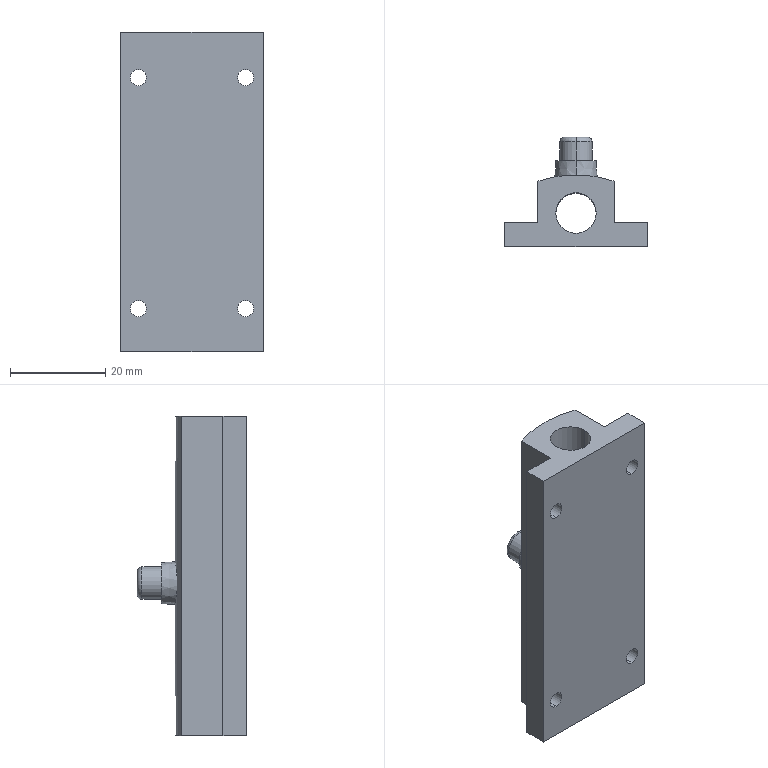Part | SolidWorks | features ICE 4, Extrusion 1, Fillet 1, HoleWzd 1 | 2 solids | 41 faces | box 30 x 23 x 67 mm | volume 16541 mm3 | cylinder 15 | plane 14 | cone 10 | torus 2 | commonest cylinder face diameters 3.4 x8 6.8 x2 7 x2 8.5 x2 50 x1
STEP:
#1=CARTESIAN_POINT('',(-4.25,7.,-33.5));
#2=VERTEX_POINT('',#1);
#3=CARTESIAN_POINT('',(4.25,7.,-33.5));
#4=VERTEX_POINT('',#3);
#5=CARTESIAN_POINT('',(0.,7.,-33.5));
#6=DIRECTION('',(0.,0.,1.));
#7=DIRECTION('',(1.,0.,0.));
#8=AXIS2_PLACEMENT_3D('',#5,#6,#7);
#9=CIRCLE('',#8,4.25);
#10=EDGE_CURVE('',#2,#4,#9,.T.);
#11=ORIENTED_EDGE('',*,*,#10,.F.);
#12=CARTESIAN_POINT('',(-4.25,7.,33.5));
#13=VERTEX_POINT('',#12);
#14=CARTESIAN_POINT('',(-4.25,7.,-33.5));
#15=DIRECTION('',(0.,0.,1.));
#16=VECTOR('',#15,1000.);
#17=LINE('',#14,#16);
#18=EDGE_CURVE('',#2,#13,#17,.T.);
#19=ORIENTED_EDGE('',*,*,#18,.T.);
#20=CARTESIAN_POINT('',(4.25,7.,33.5));
#21=VERTEX_POINT('',#20);
#22=CARTESIAN_POINT('',(0.,7.,33.5));
#23=DIRECTION('',(0.,0.,1.));
#24=DIRECTION('',(1.,0.,0.));
#25=AXIS2_PLACEMENT_3D('',#22,#23,#24);
#26=CIRCLE('',#25,4.25);
#27=EDGE_CURVE('',#13,#21,#26,.T.);
#28=ORIENTED_EDGE('',*,*,#27,.T.);
#29=CARTESIAN_POINT('',(4.25,7.,-33.5));
#30=DIRECTION('',(0.,0.,1.));
#31=VECTOR('',#30,1000.);
#32=LINE('',#29,#31);
#33=EDGE_CURVE('',#4,#21,#32,.T.);
#34=ORIENTED_EDGE('',*,*,#33,.F.);
#35=EDGE_LOOP('',(#11,#19,#28,#34));
#36=FACE_OUTER_BOUND('',#35,.T.);
#37=CARTESIAN_POINT('',(0.,7.,-33.5));
#38=DIRECTION('',(0.,0.,1.));
#39=DIRECTION('',(1.,0.,0.));
#40=AXIS2_PLACEMENT_3D('',#37,#38,#39);
#41=CYLINDRICAL_SURFACE('',#40,4.25);
#42=ADVANCED_FACE('',(#36),#41,.F.);
#43=CARTESIAN_POINT('',(-1.436,11.,-4.692));
#44=VERTEX_POINT('',#43);
#45=CARTESIAN_POINT('',(0.,11.25,-5.));
#46=VERTEX_POINT('',#45);
#47=CARTESIAN_POINT('',(-1.436,11.,-4.692));
#48=CARTESIAN_POINT('',(-1.217,11.079,-4.791));
#49=CARTESIAN_POINT('',(-0.9864,11.141,-4.867));
#50=CARTESIAN_POINT('',(-0.6235,11.206,-4.946));
#51=CARTESIAN_POINT('',(-0.4987,11.222,-4.967));
#52=CARTESIAN_POINT('',(-0.2496,11.245,-4.993));
#53=CARTESIAN_POINT('',(-0.1249,11.25,-5.));
#54=CARTESIAN_POINT('',(0.,11.25,-5.));
#55=B_SPLINE_CURVE_WITH_KNOTS('',3,(#47,#48,#49,#50,#51,#52,#53,#54),.UNSPECIFIED.,.F.,.F.,(4,2,2,4),(0.,0.0007508,0.001126,0.001502),.UNSPECIFIED.);
#56=EDGE_CURVE('',#44,#46,#55,.T.);
#57=ORIENTED_EDGE('',*,*,#56,.T.);
#58=CARTESIAN_POINT('',(0.,18.,-5.));
#59=VERTEX_POINT('',#58);
#60=CARTESIAN_POINT('',(0.,11.,-5.));
#61=DIRECTION('',(0.,1.,0.));
#62=VECTOR('',#61,1000.);
#63=LINE('',#60,#62);
#64=EDGE_CURVE('',#46,#59,#63,.T.);
#65=ORIENTED_EDGE('',*,*,#64,.T.);
#66=CARTESIAN_POINT('',(0.,18.,2.));
#67=VERTEX_POINT('',#66);
#68=CARTESIAN_POINT('',(0.,18.,-1.5));
#69=DIRECTION('',(0.,1.,0.));
#70=DIRECTION('',(0.,0.,1.));
#71=AXIS2_PLACEMENT_3D('',#68,#69,#70);
#72=CIRCLE('',#71,3.5);
#73=EDGE_CURVE('',#59,#67,#72,.T.);
#74=ORIENTED_EDGE('',*,*,#73,.T.);
#75=CARTESIAN_POINT('',(0.,11.25,2.));
#76=VERTEX_POINT('',#75);
#77=CARTESIAN_POINT('',(0.,11.,2.));
#78=DIRECTION('',(0.,1.,0.));
#79=VECTOR('',#78,1000.);
#80=LINE('',#77,#79);
#81=EDGE_CURVE('',#76,#67,#80,.T.);
#82=ORIENTED_EDGE('',*,*,#81,.F.);
#83=CARTESIAN_POINT('',(-1.436,11.,1.692));
#84=VERTEX_POINT('',#83);
#85=CARTESIAN_POINT('',(0.,11.25,2.));
#86=CARTESIAN_POINT('',(-0.2494,11.25,2.));
#87=CARTESIAN_POINT('',(-0.5029,11.227,1.972));
#88=CARTESIAN_POINT('',(-0.9847,11.142,1.868));
#89=CARTESIAN_POINT('',(-1.217,11.079,1.79));
#90=CARTESIAN_POINT('',(-1.436,11.,1.692));
#91=B_SPLINE_CURVE_WITH_KNOTS('',3,(#85,#86,#87,#88,#89,#90),.UNSPECIFIED.,.F.,.F.,(4,2,4),(0.001502,0.002251,0.003),.UNSPECIFIED.);
#92=EDGE_CURVE('',#76,#84,#91,.T.);
#93=ORIENTED_EDGE('',*,*,#92,.T.);
#94=CARTESIAN_POINT('',(0.,11.,-1.5));
#95=DIRECTION('',(0.,1.,0.));
#96=DIRECTION('',(0.,0.,1.));
#97=AXIS2_PLACEMENT_3D('',#94,#95,#96);
#98=CIRCLE('',#97,3.5);
#99=EDGE_CURVE('',#44,#84,#98,.T.);
#100=ORIENTED_EDGE('',*,*,#99,.F.);
#101=EDGE_LOOP('',(#57,#65,#74,#82,#93,#100));
#102=FACE_OUTER_BOUND('',#101,.T.);
#103=CARTESIAN_POINT('',(0.,11.,-1.5));
#104=DIRECTION('',(0.,1.,0.));
#105=DIRECTION('',(0.,0.,1.));
#106=AXIS2_PLACEMENT_3D('',#103,#104,#105);
#107=CYLINDRICAL_SURFACE('',#106,3.5);
#108=ADVANCED_FACE('',(#102),#107,.F.);
#109=CARTESIAN_POINT('',(0.,18.,-5.819));
#110=VERTEX_POINT('',#109);
#111=CARTESIAN_POINT('',(0.,18.,2.819));
#112=VERTEX_POINT('',#111);
#113=CARTESIAN_POINT('',(0.,18.,-1.5));
#114=DIRECTION('',(0.,1.,0.));
#115=DIRECTION('',(0.,0.,1.));
#116=AXIS2_PLACEMENT_3D('',#113,#114,#115);
#117=CIRCLE('',#116,4.319);
#118=EDGE_CURVE('',#110,#112,#117,.T.);
#119=ORIENTED_EDGE('',*,*,#118,.F.);
#120=CARTESIAN_POINT('',(0.,15.,-5.976));
#121=VERTEX_POINT('',#120);
#122=CARTESIAN_POINT('',(0.,5.,-6.5));
#123=DIRECTION('',(0.,-0.9986,-0.05234));
#124=VECTOR('',#123,1000.);
#125=LINE('',#122,#124);
#126=EDGE_CURVE('',#110,#121,#125,.T.);
#127=ORIENTED_EDGE('',*,*,#126,.T.);
#128=CARTESIAN_POINT('',(0.,15.,2.976));
#129=VERTEX_POINT('',#128);
#130=CARTESIAN_POINT('',(0.,15.,-5.976));
#131=CARTESIAN_POINT('',(-0.293,15.,-5.976));
#132=CARTESIAN_POINT('',(-0.5848,14.995,-5.948));
#133=CARTESIAN_POINT('',(-1.166,14.974,-5.833));
#134=CARTESIAN_POINT('',(-1.448,14.96,-5.748));
#135=CARTESIAN_POINT('',(-1.988,14.922,-5.525));
#136=CARTESIAN_POINT('',(-2.25,14.9,-5.386));
#137=CARTESIAN_POINT('',(-2.741,14.85,-5.06));
#138=CARTESIAN_POINT('',(-2.969,14.824,-4.875));
#139=CARTESIAN_POINT('',(-3.388,14.77,-4.459));
#140=CARTESIAN_POINT('',(-3.574,14.744,-4.232));
#141=CARTESIAN_POINT('',(-3.9,14.694,-3.748));
#142=CARTESIAN_POINT('',(-4.041,14.672,-3.487));
#143=CARTESIAN_POINT('',(-4.267,14.633,-2.943));
#144=CARTESIAN_POINT('',(-4.353,14.618,-2.664));
#145=CARTESIAN_POINT('',(-4.468,14.598,-2.088));
#146=CARTESIAN_POINT('',(-4.497,14.592,-1.79));
#147=CARTESIAN_POINT('',(-4.497,14.592,-1.204));
#148=CARTESIAN_POINT('',(-4.468,14.598,-0.9123));
#149=CARTESIAN_POINT('',(-4.352,14.618,-0.3332));
#150=CARTESIAN_POINT('',(-4.265,14.634,-0.04984));
#151=CARTESIAN_POINT('',(-4.039,14.672,0.4895));
#152=CARTESIAN_POINT('',(-3.899,14.695,0.7498));
#153=CARTESIAN_POINT('',(-3.57,14.744,1.238));
#154=CARTESIAN_POINT('',(-3.383,14.771,1.463));
#155=CARTESIAN_POINT('',(-2.969,14.824,1.875));
#156=CARTESIAN_POINT('',(-2.738,14.851,2.063));
#157=CARTESIAN_POINT('',(-2.25,14.9,2.386));
#158=CARTESIAN_POINT('',(-1.992,14.922,2.523));
#159=CARTESIAN_POINT('',(-1.448,14.96,2.748));
#160=CARTESIAN_POINT('',(-1.163,14.975,2.833));
#161=CARTESIAN_POINT('',(-0.589,14.995,2.947));
#162=CARTESIAN_POINT('',(-0.297,15.,2.976));
#163=CARTESIAN_POINT('',(0.,15.,2.976));
#164=B_SPLINE_CURVE_WITH_KNOTS('',3,(#130,#131,#132,#133,#134,#135,#136,#137,#138,#139,#140,#141,#142,#143,#144,#145,#146,#147,#148,#149,#150,#151,#152,#153,#154,#155,#156,#157,#158,#159,#160,#161,#162,#163),.UNSPECIFIED.,.F.,.F.,(4,2,2,2,2,2,2,2,2,2,2,2,2,2,2,2,4),(0.02455,0.02543,0.02631,0.02719,0.02807,0.02894,0.02982,0.0307,0.03158,0.03246,0.03334,0.03421,0.03509,0.03597,0.03685,0.03773,0.03861),.UNSPECIFIED.);
#165=EDGE_CURVE('',#121,#129,#164,.T.);
#166=ORIENTED_EDGE('',*,*,#165,.T.);
#167=CARTESIAN_POINT('',(0.,5.,3.5));
#168=DIRECTION('',(0.,-0.9986,0.05234));
#169=VECTOR('',#168,1000.);
#170=LINE('',#167,#169);
#171=EDGE_CURVE('',#112,#129,#170,.T.);
#172=ORIENTED_EDGE('',*,*,#171,.F.);
#173=EDGE_LOOP('',(#119,#127,#166,#172));
#174=FACE_OUTER_BOUND('',#173,.T.);
#175=CARTESIAN_POINT('',(0.,5.,-1.5));
#176=DIRECTION('',(0.,-1.,0.));
#177=DIRECTION('',(0.,0.,1.));
#178=AXIS2_PLACEMENT_3D('',#175,#176,#177);
#179=CONICAL_SURFACE('',#178,5.,0.05236);
#180=ADVANCED_FACE('',(#174),#179,.T.);
#181=CARTESIAN_POINT('',(-11.25,3.5,-26.2));
#182=VERTEX_POINT('',#181);
#183=CARTESIAN_POINT('',(-11.25,3.5,-22.8));
#184=VERTEX_POINT('',#183);
#185=CARTESIAN_POINT('',(-11.25,3.5,-24.5));
#186=DIRECTION('',(0.,1.,0.));
#187=DIRECTION('',(0.,0.,1.));
#188=AXIS2_PLACEMENT_3D('',#185,#186,#187);
#189=CIRCLE('',#188,1.7);
#190=EDGE_CURVE('',#182,#184,#189,.T.);
#191=ORIENTED_EDGE('',*,*,#190,.F.);
#192=CARTESIAN_POINT('',(-11.25,5.,-27.7));
#193=VERTEX_POINT('',#192);
#194=CARTESIAN_POINT('',(-11.25,5.,-27.7));
#195=DIRECTION('',(0.,0.7071,-0.7071));
#196=VECTOR('',#195,1000.);
#197=LINE('',#194,#196);
#198=EDGE_CURVE('',#182,#193,#197,.T.);
#199=ORIENTED_EDGE('',*,*,#198,.T.);
#200=CARTESIAN_POINT('',(-11.25,5.,-21.3));
#201=VERTEX_POINT('',#200);
#202=CARTESIAN_POINT('',(-11.25,5.,-24.5));
#203=DIRECTION('',(0.,1.,0.));
#204=DIRECTION('',(0.,0.,1.));
#205=AXIS2_PLACEMENT_3D('',#202,#203,#204);
#206=CIRCLE('',#205,3.2);
#207=EDGE_CURVE('',#193,#201,#206,.T.);
#208=ORIENTED_EDGE('',*,*,#207,.T.);
#209=CARTESIAN_POINT('',(-11.25,5.,-21.3));
#210=DIRECTION('',(0.,0.7071,0.7071));
#211=VECTOR('',#210,1000.);
#212=LINE('',#209,#211);
#213=EDGE_CURVE('',#184,#201,#212,.T.);
#214=ORIENTED_EDGE('',*,*,#213,.F.);
#215=EDGE_LOOP('',(#191,#199,#208,#214));
#216=FACE_OUTER_BOUND('',#215,.T.);
#217=CARTESIAN_POINT('',(-11.25,5.,-24.5));
#218=DIRECTION('',(0.,1.,0.));
#219=DIRECTION('',(0.,0.,1.));
#220=AXIS2_PLACEMENT_3D('',#217,#218,#219);
#221=CONICAL_SURFACE('',#220,3.2,0.7854);
#222=ADVANCED_FACE('',(#216),#221,.F.);
#223=CARTESIAN_POINT('',(-11.25,0.,-26.2));
#224=VERTEX_POINT('',#223);
#225=CARTESIAN_POINT('',(-11.25,0.,-22.8));
#226=VERTEX_POINT('',#225);
#227=CARTESIAN_POINT('',(-11.25,0.,-24.5));
#228=DIRECTION('',(0.,1.,0.));
#229=DIRECTION('',(0.,0.,1.));
#230=AXIS2_PLACEMENT_3D('',#227,#228,#229);
#231=CIRCLE('',#230,1.7);
#232=EDGE_CURVE('',#224,#226,#231,.T.);
#233=ORIENTED_EDGE('',*,*,#232,.F.);
#234=CARTESIAN_POINT('',(-11.25,5.,-26.2));
#235=DIRECTION('',(0.,1.,0.));
#236=VECTOR('',#235,1000.);
#237=LINE('',#234,#236);
#238=EDGE_CURVE('',#224,#182,#237,.T.);
#239=ORIENTED_EDGE('',*,*,#238,.T.);
#240=ORIENTED_EDGE('',*,*,#190,.T.);
#241=CARTESIAN_POINT('',(-11.25,5.,-22.8));
#242=DIRECTION('',(0.,1.,0.));
#243=VECTOR('',#242,1000.);
#244=LINE('',#241,#243);
#245=EDGE_CURVE('',#226,#184,#244,.T.);
#246=ORIENTED_EDGE('',*,*,#245,.F.);
#247=EDGE_LOOP('',(#233,#239,#240,#246));
#248=FACE_OUTER_BOUND('',#247,.T.);
#249=CARTESIAN_POINT('',(-11.25,5.,-24.5));
#250=DIRECTION('',(0.,1.,0.));
#251=DIRECTION('',(0.,0.,1.));
#252=AXIS2_PLACEMENT_3D('',#249,#250,#251);
#253=CYLINDRICAL_SURFACE('',#252,1.7);
#254=ADVANCED_FACE('',(#248),#253,.F.);
#255=CARTESIAN_POINT('',(-11.25,3.5,22.3));
#256=VERTEX_POINT('',#255);
#257=CARTESIAN_POINT('',(-11.25,3.5,25.7));
#258=VERTEX_POINT('',#257);
#259=CARTESIAN_POINT('',(-11.25,3.5,24.));
#260=DIRECTION('',(0.,1.,0.));
#261=DIRECTION('',(0.,0.,1.));
#262=AXIS2_PLACEMENT_3D('',#259,#260,#261);
#263=CIRCLE('',#262,1.7);
#264=EDGE_CURVE('',#256,#258,#263,.T.);
#265=ORIENTED_EDGE('',*,*,#264,.F.);
#266=CARTESIAN_POINT('',(-11.25,5.,20.8));
#267=VERTEX_POINT('',#266);
#268=CARTESIAN_POINT('',(-11.25,5.,20.8));
#269=DIRECTION('',(0.,0.7071,-0.7071));
#270=VECTOR('',#269,1000.);
#271=LINE('',#268,#270);
#272=EDGE_CURVE('',#256,#267,#271,.T.);
#273=ORIENTED_EDGE('',*,*,#272,.T.);
#274=CARTESIAN_POINT('',(-11.25,5.,27.2));
#275=VERTEX_POINT('',#274);
#276=CARTESIAN_POINT('',(-11.25,5.,24.));
#277=DIRECTION('',(0.,1.,0.));
#278=DIRECTION('',(0.,0.,1.));
#279=AXIS2_PLACEMENT_3D('',#276,#277,#278);
#280=CIRCLE('',#279,3.2);
#281=EDGE_CURVE('',#267,#275,#280,.T.);
#282=ORIENTED_EDGE('',*,*,#281,.T.);
#283=CARTESIAN_POINT('',(-11.25,5.,27.2));
#284=DIRECTION('',(0.,0.7071,0.7071));
#285=VECTOR('',#284,1000.);
#286=LINE('',#283,#285);
#287=EDGE_CURVE('',#258,#275,#286,.T.);
#288=ORIENTED_EDGE('',*,*,#287,.F.);
#289=EDGE_LOOP('',(#265,#273,#282,#288));
#290=FACE_OUTER_BOUND('',#289,.T.);
#291=CARTESIAN_POINT('',(-11.25,5.,24.));
#292=DIRECTION('',(0.,1.,0.));
#293=DIRECTION('',(0.,0.,1.));
#294=AXIS2_PLACEMENT_3D('',#291,#292,#293);
#295=CONICAL_SURFACE('',#294,3.2,0.7854);
#296=ADVANCED_FACE('',(#290),#295,.F.);
#297=CARTESIAN_POINT('',(-11.25,0.,22.3));
#298=VERTEX_POINT('',#297);
#299=CARTESIAN_POINT('',(-11.25,0.,25.7));
#300=VERTEX_POINT('',#299);
#301=CARTESIAN_POINT('',(-11.25,0.,24.));
#302=DIRECTION('',(0.,1.,0.));
#303=DIRECTION('',(0.,0.,1.));
#304=AXIS2_PLACEMENT_3D('',#301,#302,#303);
#305=CIRCLE('',#304,1.7);
#306=EDGE_CURVE('',#298,#300,#305,.T.);
#307=ORIENTED_EDGE('',*,*,#306,.F.);
#308=CARTESIAN_POINT('',(-11.25,5.,22.3));
#309=DIRECTION('',(0.,1.,0.));
#310=VECTOR('',#309,1000.);
#311=LINE('',#308,#310);
#312=EDGE_CURVE('',#298,#256,#311,.T.);
#313=ORIENTED_EDGE('',*,*,#312,.T.);
#314=ORIENTED_EDGE('',*,*,#264,.T.);
#315=CARTESIAN_POINT('',(-11.25,5.,25.7));
#316=DIRECTION('',(0.,1.,0.));
#317=VECTOR('',#316,1000.);
#318=LINE('',#315,#317);
#319=EDGE_CURVE('',#300,#258,#318,.T.);
#320=ORIENTED_EDGE('',*,*,#319,.F.);
#321=EDGE_LOOP('',(#307,#313,#314,#320));
#322=FACE_OUTER_BOUND('',#321,.T.);
#323=CARTESIAN_POINT('',(-11.25,5.,24.));
#324=DIRECTION('',(0.,1.,0.));
#325=DIRECTION('',(0.,0.,1.));
#326=AXIS2_PLACEMENT_3D('',#323,#324,#325);
#327=CYLINDRICAL_SURFACE('',#326,1.7);
#328=ADVANCED_FACE('',(#322),#327,.F.);
#329=CARTESIAN_POINT('',(11.25,3.5,22.3));
#330=VERTEX_POINT('',#329);
#331=CARTESIAN_POINT('',(11.25,3.5,25.7));
#332=VERTEX_POINT('',#331);
#333=CARTESIAN_POINT('',(11.25,3.5,24.));
#334=DIRECTION('',(0.,1.,0.));
#335=DIRECTION('',(0.,0.,1.));
#336=AXIS2_PLACEMENT_3D('',#333,#334,#335);
#337=CIRCLE('',#336,1.7);
#338=EDGE_CURVE('',#330,#332,#337,.T.);
#339=ORIENTED_EDGE('',*,*,#338,.F.);
#340=CARTESIAN_POINT('',(11.25,5.,20.8));
#341=VERTEX_POINT('',#340);
#342=CARTESIAN_POINT('',(11.25,5.,20.8));
#343=DIRECTION('',(0.,0.7071,-0.7071));
#344=VECTOR('',#343,1000.);
#345=LINE('',#342,#344);
#346=EDGE_CURVE('',#330,#341,#345,.T.);
#347=ORIENTED_EDGE('',*,*,#346,.T.);
#348=CARTESIAN_POINT('',(11.25,5.,27.2));
#349=VERTEX_POINT('',#348);
#350=CARTESIAN_POINT('',(11.25,5.,24.));
#351=DIRECTION('',(0.,1.,0.));
#352=DIRECTION('',(0.,0.,1.));
#353=AXIS2_PLACEMENT_3D('',#350,#351,#352);
#354=CIRCLE('',#353,3.2);
#355=EDGE_CURVE('',#341,#349,#354,.T.);
#356=ORIENTED_EDGE('',*,*,#355,.T.);
#357=CARTESIAN_POINT('',(11.25,5.,27.2));
#358=DIRECTION('',(0.,0.7071,0.7071));
#359=VECTOR('',#358,1000.);
#360=LINE('',#357,#359);
#361=EDGE_CURVE('',#332,#349,#360,.T.);
#362=ORIENTED_EDGE('',*,*,#361,.F.);
#363=EDGE_LOOP('',(#339,#347,#356,#362));
#364=FACE_OUTER_BOUND('',#363,.T.);
#365=CARTESIAN_POINT('',(11.25,5.,24.));
#366=DIRECTION('',(0.,1.,0.));
#367=DIRECTION('',(0.,0.,1.));
#368=AXIS2_PLACEMENT_3D('',#365,#366,#367);
#369=CONICAL_SURFACE('',#368,3.2,0.7854);
#370=ADVANCED_FACE('',(#364),#369,.F.);
#371=CARTESIAN_POINT('',(11.25,0.,22.3));
#372=VERTEX_POINT('',#371);
#373=CARTESIAN_POINT('',(11.25,0.,25.7));
#374=VERTEX_POINT('',#373);
#375=CARTESIAN_POINT('',(11.25,0.,24.));
#376=DIRECTION('',(0.,1.,0.));
#377=DIRECTION('',(0.,0.,1.));
#378=AXIS2_PLACEMENT_3D('',#375,#376,#377);
#379=CIRCLE('',#378,1.7);
#380=EDGE_CURVE('',#372,#374,#379,.T.);
#381=ORIENTED_EDGE('',*,*,#380,.F.);
#382=CARTESIAN_POINT('',(11.25,5.,22.3));
#383=DIRECTION('',(0.,1.,0.));
#384=VECTOR('',#383,1000.);
#385=LINE('',#382,#384);
#386=EDGE_CURVE('',#372,#330,#385,.T.);
#387=ORIENTED_EDGE('',*,*,#386,.T.);
#388=ORIENTED_EDGE('',*,*,#338,.T.);
#389=CARTESIAN_POINT('',(11.25,5.,25.7));
#390=DIRECTION('',(0.,1.,0.));
#391=VECTOR('',#390,1000.);
#392=LINE('',#389,#391);
#393=EDGE_CURVE('',#374,#332,#392,.T.);
#394=ORIENTED_EDGE('',*,*,#393,.F.);
#395=EDGE_LOOP('',(#381,#387,#388,#394));
#396=FACE_OUTER_BOUND('',#395,.T.);
#397=CARTESIAN_POINT('',(11.25,5.,24.));
#398=DIRECTION('',(0.,1.,0.));
#399=DIRECTION('',(0.,0.,1.));
#400=AXIS2_PLACEMENT_3D('',#397,#398,#399);
#401=CYLINDRICAL_SURFACE('',#400,1.7);
#402=ADVANCED_FACE('',(#396),#401,.F.);
#403=CARTESIAN_POINT('',(11.25,3.5,-26.2));
#404=VERTEX_POINT('',#403);
#405=CARTESIAN_POINT('',(11.25,3.5,-22.8));
#406=VERTEX_POINT('',#405);
#407=CARTESIAN_POINT('',(11.25,3.5,-24.5));
#408=DIRECTION('',(0.,1.,0.));
#409=DIRECTION('',(0.,0.,1.));
#410=AXIS2_PLACEMENT_3D('',#407,#408,#409);
#411=CIRCLE('',#410,1.7);
#412=EDGE_CURVE('',#404,#406,#411,.T.);
#413=ORIENTED_EDGE('',*,*,#412,.F.);
#414=CARTESIAN_POINT('',(11.25,5.,-27.7));
#415=VERTEX_POINT('',#414);
#416=CARTESIAN_POINT('',(11.25,5.,-27.7));
#417=DIRECTION('',(0.,0.7071,-0.7071));
#418=VECTOR('',#417,1000.);
#419=LINE('',#416,#418);
#420=EDGE_CURVE('',#404,#415,#419,.T.);
#421=ORIENTED_EDGE('',*,*,#420,.T.);
#422=CARTESIAN_POINT('',(11.25,5.,-21.3));
#423=VERTEX_POINT('',#422);
#424=CARTESIAN_POINT('',(11.25,5.,-24.5));
#425=DIRECTION('',(0.,1.,0.));
#426=DIRECTION('',(0.,0.,1.));
#427=AXIS2_PLACEMENT_3D('',#424,#425,#426);
#428=CIRCLE('',#427,3.2);
#429=EDGE_CURVE('',#415,#423,#428,.T.);
#430=ORIENTED_EDGE('',*,*,#429,.T.);
#431=CARTESIAN_POINT('',(11.25,5.,-21.3));
#432=DIRECTION('',(0.,0.7071,0.7071));
#433=VECTOR('',#432,1000.);
#434=LINE('',#431,#433);
#435=EDGE_CURVE('',#406,#423,#434,.T.);
#436=ORIENTED_EDGE('',*,*,#435,.F.);
#437=EDGE_LOOP('',(#413,#421,#430,#436));
#438=FACE_OUTER_BOUND('',#437,.T.);
#439=CARTESIAN_POINT('',(11.25,5.,-24.5));
#440=DIRECTION('',(0.,1.,0.));
#441=DIRECTION('',(0.,0.,1.));
#442=AXIS2_PLACEMENT_3D('',#439,#440,#441);
#443=CONICAL_SURFACE('',#442,3.2,0.7854);
#444=ADVANCED_FACE('',(#438),#443,.F.);
#445=CARTESIAN_POINT('',(11.25,0.,-26.2));
#446=VERTEX_POINT('',#445);
#447=CARTESIAN_POINT('',(11.25,0.,-22.8));
#448=VERTEX_POINT('',#447);
#449=CARTESIAN_POINT('',(11.25,0.,-24.5));
#450=DIRECTION('',(0.,1.,0.));
#451=DIRECTION('',(0.,0.,1.));
#452=AXIS2_PLACEMENT_3D('',#449,#450,#451);
#453=CIRCLE('',#452,1.7);
#454=EDGE_CURVE('',#446,#448,#453,.T.);
#455=ORIENTED_EDGE('',*,*,#454,.F.);
#456=CARTESIAN_POINT('',(11.25,5.,-26.2));
#457=DIRECTION('',(0.,1.,0.));
#458=VECTOR('',#457,1000.);
#459=LINE('',#456,#458);
#460=EDGE_CURVE('',#446,#404,#459,.T.);
#461=ORIENTED_EDGE('',*,*,#460,.T.);
#462=ORIENTED_EDGE('',*,*,#412,.T.);
#463=CARTESIAN_POINT('',(11.25,5.,-22.8));
#464=DIRECTION('',(0.,1.,0.));
#465=VECTOR('',#464,1000.);
#466=LINE('',#463,#465);
#467=EDGE_CURVE('',#448,#406,#466,.T.);
#468=ORIENTED_EDGE('',*,*,#467,.F.);
#469=EDGE_LOOP('',(#455,#461,#462,#468));
#470=FACE_OUTER_BOUND('',#469,.T.);
#471=CARTESIAN_POINT('',(11.25,5.,-24.5));
#472=DIRECTION('',(0.,1.,0.));
#473=DIRECTION('',(0.,0.,1.));
#474=AXIS2_PLACEMENT_3D('',#471,#472,#473);
#475=CYLINDRICAL_SURFACE('',#474,1.7);
#476=ADVANCED_FACE('',(#470),#475,.F.);
#477=CARTESIAN_POINT('',(-1.436,11.,-33.5));
#478=DIRECTION('',(0.,0.,1.));
#479=VECTOR('',#478,1000.);
#480=LINE('',#477,#479);
#481=EDGE_CURVE('',#44,#84,#480,.T.);
#482=ORIENTED_EDGE('',*,*,#481,.F.);
#483=ORIENTED_EDGE('',*,*,#99,.T.);
#484=EDGE_LOOP('',(#482,#483));
#485=FACE_OUTER_BOUND('',#484,.T.);
#486=CARTESIAN_POINT('',(0.,11.,-1.5));
#487=DIRECTION('',(0.,1.,0.));
#488=DIRECTION('',(0.,0.,1.));
#489=AXIS2_PLACEMENT_3D('',#486,#487,#488);
#490=PLANE('',#489);
#491=ADVANCED_FACE('',(#485),#490,.T.);
#492=CARTESIAN_POINT('',(8.,13.685,-33.5));
#493=VERTEX_POINT('',#492);
#494=CARTESIAN_POINT('',(-8.,13.685,-33.5));
#495=VERTEX_POINT('',#494);
#496=CARTESIAN_POINT('',(0.,-10.,-33.5));
#497=DIRECTION('',(0.,0.,1.));
#498=DIRECTION('',(-1.,0.,0.));
#499=AXIS2_PLACEMENT_3D('',#496,#497,#498);
#500=CIRCLE('',#499,25.);
#501=EDGE_CURVE('',#493,#495,#500,.T.);
#502=ORIENTED_EDGE('',*,*,#501,.T.);
#503=CARTESIAN_POINT('',(-8.,13.685,33.5));
#504=VERTEX_POINT('',#503);
#505=CARTESIAN_POINT('',(-8.,13.685,33.5));
#506=DIRECTION('',(0.,0.,-1.));
#507=VECTOR('',#506,1000.);
#508=LINE('',#505,#507);
#509=EDGE_CURVE('',#504,#495,#508,.T.);
#510=ORIENTED_EDGE('',*,*,#509,.F.);
#511=CARTESIAN_POINT('',(8.,13.685,33.5));
#512=VERTEX_POINT('',#511);
#513=CARTESIAN_POINT('',(0.,-10.,33.5));
#514=DIRECTION('',(0.,0.,1.));
#515=DIRECTION('',(-1.,0.,0.));
#516=AXIS2_PLACEMENT_3D('',#513,#514,#515);
#517=CIRCLE('',#516,25.);
#518=EDGE_CURVE('',#512,#504,#517,.T.);
#519=ORIENTED_EDGE('',*,*,#518,.F.);
#520=CARTESIAN_POINT('',(8.,13.685,33.5));
#521=DIRECTION('',(0.,0.,-1.));
#522=VECTOR('',#521,1000.);
#523=LINE('',#520,#522);
#524=EDGE_CURVE('',#512,#493,#523,.T.);
#525=ORIENTED_EDGE('',*,*,#524,.T.);
#526=EDGE_LOOP('',(#502,#510,#519,#525));
#527=FACE_OUTER_BOUND('',#526,.T.);
#528=CARTESIAN_POINT('',(0.,15.,2.976));
#529=CARTESIAN_POINT('',(0.297,15.,2.976));
#530=CARTESIAN_POINT('',(0.589,14.995,2.947));
#531=CARTESIAN_POINT('',(1.164,14.975,2.833));
#532=CARTESIAN_POINT('',(1.449,14.959,2.747));
#533=CARTESIAN_POINT('',(1.993,14.922,2.523));
#534=CARTESIAN_POINT('',(2.251,14.9,2.386));
#535=CARTESIAN_POINT('',(2.739,14.851,2.062));
#536=CARTESIAN_POINT('',(2.97,14.824,1.874));
#537=CARTESIAN_POINT('',(3.384,14.771,1.462));
#538=CARTESIAN_POINT('',(3.57,14.744,1.237));
#539=CARTESIAN_POINT('',(3.9,14.695,0.7484));
#540=CARTESIAN_POINT('',(4.04,14.672,0.4884));
#541=CARTESIAN_POINT('',(4.265,14.634,-0.05062));
#542=CARTESIAN_POINT('',(4.352,14.618,-0.3337));
#543=CARTESIAN_POINT('',(4.468,14.598,-0.9132));
#544=CARTESIAN_POINT('',(4.497,14.592,-1.205));
#545=CARTESIAN_POINT('',(4.497,14.592,-1.791));
#546=CARTESIAN_POINT('',(4.468,14.598,-2.089));
#547=CARTESIAN_POINT('',(4.352,14.618,-2.665));
#548=CARTESIAN_POINT('',(4.267,14.633,-2.945));
#549=CARTESIAN_POINT('',(4.04,14.672,-3.488));
#550=CARTESIAN_POINT('',(3.899,14.695,-3.75));
#551=CARTESIAN_POINT('',(3.573,14.744,-4.234));
#552=CARTESIAN_POINT('',(3.385,14.771,-4.461));
#553=CARTESIAN_POINT('',(2.967,14.824,-4.877));
#554=CARTESIAN_POINT('',(2.74,14.851,-5.061));
#555=CARTESIAN_POINT('',(2.254,14.899,-5.384));
#556=CARTESIAN_POINT('',(1.99,14.922,-5.524));
#557=CARTESIAN_POINT('',(1.447,14.96,-5.748));
#558=CARTESIAN_POINT('',(1.167,14.974,-5.832));
#559=CARTESIAN_POINT('',(0.5907,14.995,-5.947));
#560=CARTESIAN_POINT('',(0.2931,15.,-5.976));
#561=CARTESIAN_POINT('',(0.,15.,-5.976));
#562=B_SPLINE_CURVE_WITH_KNOTS('',3,(#528,#529,#530,#531,#532,#533,#534,#535,#536,#537,#538,#539,#540,#541,#542,#543,#544,#545,#546,#547,#548,#549,#550,#551,#552,#553,#554,#555,#556,#557,#558,#559,#560,#561),.UNSPECIFIED.,.F.,.F.,(4,2,2,2,2,2,2,2,2,2,2,2,2,2,2,2,4),(0.01049,0.01137,0.01225,0.01313,0.01401,0.01489,0.01577,0.01664,0.01752,0.0184,0.01928,0.02016,0.02104,0.02192,0.02279,0.02367,0.02455),.UNSPECIFIED.);
#563=EDGE_CURVE('',#129,#121,#562,.T.);
#564=ORIENTED_EDGE('',*,*,#563,.F.);
#565=ORIENTED_EDGE('',*,*,#165,.F.);
#566=EDGE_LOOP('',(#564,#565));
#567=FACE_BOUND('',#566,.T.);
#568=CARTESIAN_POINT('',(0.,-10.,33.5));
#569=DIRECTION('',(0.,0.,-1.));
#570=DIRECTION('',(-1.,0.,0.));
#571=AXIS2_PLACEMENT_3D('',#568,#569,#570);
#572=CYLINDRICAL_SURFACE('',#571,25.);
#573=ADVANCED_FACE('',(#527,#567),#572,.T.);
#574=CARTESIAN_POINT('',(15.,0.,-33.5));
#575=VERTEX_POINT('',#574);
#576=CARTESIAN_POINT('',(15.,5.,-33.5));
#577=VERTEX_POINT('',#576);
#578=CARTESIAN_POINT('',(15.,5.,-33.5));
#579=DIRECTION('',(0.,1.,0.));
#580=VECTOR('',#579,1000.);
#581=LINE('',#578,#580);
#582=EDGE_CURVE('',#575,#577,#581,.T.);
#583=ORIENTED_EDGE('',*,*,#582,.T.);
#584=CARTESIAN_POINT('',(15.,5.,33.5));
#585=VERTEX_POINT('',#584);
#586=CARTESIAN_POINT('',(15.,5.,33.5));
#587=DIRECTION('',(0.,0.,-1.));
#588=VECTOR('',#587,1000.);
#589=LINE('',#586,#588);
#590=EDGE_CURVE('',#585,#577,#589,.T.);
#591=ORIENTED_EDGE('',*,*,#590,.F.);
#592=CARTESIAN_POINT('',(15.,0.,33.5));
#593=VERTEX_POINT('',#592);
#594=CARTESIAN_POINT('',(15.,5.,33.5));
#595=DIRECTION('',(0.,1.,0.));
#596=VECTOR('',#595,1000.);
#597=LINE('',#594,#596);
#598=EDGE_CURVE('',#593,#585,#597,.T.);
#599=ORIENTED_EDGE('',*,*,#598,.F.);
#600=CARTESIAN_POINT('',(15.,0.,33.5));
#601=DIRECTION('',(0.,0.,-1.));
#602=VECTOR('',#601,1000.);
#603=LINE('',#600,#602);
#604=EDGE_CURVE('',#593,#575,#603,.T.);
#605=ORIENTED_EDGE('',*,*,#604,.T.);
#606=EDGE_LOOP('',(#583,#591,#599,#605));
#607=FACE_OUTER_BOUND('',#606,.T.);
#608=CARTESIAN_POINT('',(15.,5.,33.5));
#609=DIRECTION('',(-1.,0.,0.));
#610=DIRECTION('',(0.,-1.,0.));
#611=AXIS2_PLACEMENT_3D('',#608,#609,#610);
#612=PLANE('',#611);
#613=ADVANCED_FACE('',(#607),#612,.F.);
#614=CARTESIAN_POINT('',(11.25,5.,24.));
#615=DIRECTION('',(0.,1.,0.));
#616=DIRECTION('',(0.,0.,1.));
#617=AXIS2_PLACEMENT_3D('',#614,#615,#616);
#618=CIRCLE('',#617,3.2);
#619=EDGE_CURVE('',#349,#341,#618,.T.);
#620=ORIENTED_EDGE('',*,*,#619,.F.);
#621=ORIENTED_EDGE('',*,*,#355,.F.);
#622=EDGE_LOOP('',(#620,#621));
#623=FACE_BOUND('',#622,.T.);
#624=CARTESIAN_POINT('',(11.25,5.,-24.5));
#625=DIRECTION('',(0.,1.,0.));
#626=DIRECTION('',(0.,0.,1.));
#627=AXIS2_PLACEMENT_3D('',#624,#625,#626);
#628=CIRCLE('',#627,3.2);
#629=EDGE_CURVE('',#423,#415,#628,.T.);
#630=ORIENTED_EDGE('',*,*,#629,.F.);
#631=ORIENTED_EDGE('',*,*,#429,.F.);
#632=EDGE_LOOP('',(#630,#631));
#633=FACE_BOUND('',#632,.T.);
#634=CARTESIAN_POINT('',(8.,5.,-33.5));
#635=VERTEX_POINT('',#634);
#636=CARTESIAN_POINT('',(15.,5.,-33.5));
#637=DIRECTION('',(-1.,0.,0.));
#638=VECTOR('',#637,1000.);
#639=LINE('',#636,#638);
#640=EDGE_CURVE('',#577,#635,#639,.T.);
#641=ORIENTED_EDGE('',*,*,#640,.T.);
#642=CARTESIAN_POINT('',(8.,5.,33.5));
#643=VERTEX_POINT('',#642);
#644=CARTESIAN_POINT('',(8.,5.,33.5));
#645=DIRECTION('',(0.,0.,-1.));
#646=VECTOR('',#645,1000.);
#647=LINE('',#644,#646);
#648=EDGE_CURVE('',#643,#635,#647,.T.);
#649=ORIENTED_EDGE('',*,*,#648,.F.);
#650=CARTESIAN_POINT('',(15.,5.,33.5));
#651=DIRECTION('',(-1.,0.,0.));
#652=VECTOR('',#651,1000.);
#653=LINE('',#650,#652);
#654=EDGE_CURVE('',#585,#643,#653,.T.);
#655=ORIENTED_EDGE('',*,*,#654,.F.);
#656=ORIENTED_EDGE('',*,*,#590,.T.);
#657=EDGE_LOOP('',(#641,#649,#655,#656));
#658=FACE_OUTER_BOUND('',#657,.T.);
#659=CARTESIAN_POINT('',(15.,5.,33.5));
#660=DIRECTION('',(0.,-1.,0.));
#661=DIRECTION('',(1.,0.,0.));
#662=AXIS2_PLACEMENT_3D('',#659,#660,#661);
#663=PLANE('',#662);
#664=ADVANCED_FACE('',(#623,#633,#658),#663,.F.);
#665=CARTESIAN_POINT('',(8.,5.,-33.5));
#666=DIRECTION('',(0.,1.,0.));
#667=VECTOR('',#666,1000.);
#668=LINE('',#665,#667);
#669=EDGE_CURVE('',#635,#493,#668,.T.);
#670=ORIENTED_EDGE('',*,*,#669,.T.);
#671=ORIENTED_EDGE('',*,*,#524,.F.);
#672=CARTESIAN_POINT('',(8.,5.,33.5));
#673=DIRECTION('',(0.,1.,0.));
#674=VECTOR('',#673,1000.);
#675=LINE('',#672,#674);
#676=EDGE_CURVE('',#643,#512,#675,.T.);
#677=ORIENTED_EDGE('',*,*,#676,.F.);
#678=ORIENTED_EDGE('',*,*,#648,.T.);
#679=EDGE_LOOP('',(#670,#671,#677,#678));
#680=FACE_OUTER_BOUND('',#679,.T.);
#681=CARTESIAN_POINT('',(8.,5.,33.5));
#682=DIRECTION('',(-1.,0.,0.));
#683=DIRECTION('',(0.,0.,1.));
#684=AXIS2_PLACEMENT_3D('',#681,#682,#683);
#685=PLANE('',#684);
#686=ADVANCED_FACE('',(#680),#685,.F.);
#687=CARTESIAN_POINT('',(-8.,5.,-33.5));
#688=VERTEX_POINT('',#687);
#689=CARTESIAN_POINT('',(-8.,5.,-33.5));
#690=DIRECTION('',(0.,-1.,0.));
#691=VECTOR('',#690,1000.);
#692=LINE('',#689,#691);
#693=EDGE_CURVE('',#495,#688,#692,.T.);
#694=ORIENTED_EDGE('',*,*,#693,.T.);
#695=CARTESIAN_POINT('',(-8.,5.,33.5));
#696=VERTEX_POINT('',#695);
#697=CARTESIAN_POINT('',(-8.,5.,33.5));
#698=DIRECTION('',(0.,0.,-1.));
#699=VECTOR('',#698,1000.);
#700=LINE('',#697,#699);
#701=EDGE_CURVE('',#696,#688,#700,.T.);
#702=ORIENTED_EDGE('',*,*,#701,.F.);
#703=CARTESIAN_POINT('',(-8.,5.,33.5));
#704=DIRECTION('',(0.,-1.,0.));
#705=VECTOR('',#704,1000.);
#706=LINE('',#703,#705);
#707=EDGE_CURVE('',#504,#696,#706,.T.);
#708=ORIENTED_EDGE('',*,*,#707,.F.);
#709=ORIENTED_EDGE('',*,*,#509,.T.);
#710=EDGE_LOOP('',(#694,#702,#708,#709));
#711=FACE_OUTER_BOUND('',#710,.T.);
#712=CARTESIAN_POINT('',(-8.,5.,33.5));
#713=DIRECTION('',(1.,0.,0.));
#714=DIRECTION('',(0.,0.,-1.));
#715=AXIS2_PLACEMENT_3D('',#712,#713,#714);
#716=PLANE('',#715);
#717=ADVANCED_FACE('',(#711),#716,.F.);
#718=CARTESIAN_POINT('',(-11.25,5.,-24.5));
#719=DIRECTION('',(0.,1.,0.));
#720=DIRECTION('',(0.,0.,1.));
#721=AXIS2_PLACEMENT_3D('',#718,#719,#720);
#722=CIRCLE('',#721,3.2);
#723=EDGE_CURVE('',#201,#193,#722,.T.);
#724=ORIENTED_EDGE('',*,*,#723,.F.);
#725=ORIENTED_EDGE('',*,*,#207,.F.);
#726=EDGE_LOOP('',(#724,#725));
#727=FACE_BOUND('',#726,.T.);
#728=CARTESIAN_POINT('',(-11.25,5.,24.));
#729=DIRECTION('',(0.,1.,0.));
#730=DIRECTION('',(0.,0.,1.));
#731=AXIS2_PLACEMENT_3D('',#728,#729,#730);
#732=CIRCLE('',#731,3.2);
#733=EDGE_CURVE('',#275,#267,#732,.T.);
#734=ORIENTED_EDGE('',*,*,#733,.F.);
#735=ORIENTED_EDGE('',*,*,#281,.F.);
#736=EDGE_LOOP('',(#734,#735));
#737=FACE_BOUND('',#736,.T.);
#738=CARTESIAN_POINT('',(-15.,5.,-33.5));
#739=VERTEX_POINT('',#738);
#740=CARTESIAN_POINT('',(-15.,5.,-33.5));
#741=DIRECTION('',(-1.,0.,0.));
#742=VECTOR('',#741,1000.);
#743=LINE('',#740,#742);
#744=EDGE_CURVE('',#688,#739,#743,.T.);
#745=ORIENTED_EDGE('',*,*,#744,.T.);
#746=CARTESIAN_POINT('',(-15.,5.,33.5));
#747=VERTEX_POINT('',#746);
#748=CARTESIAN_POINT('',(-15.,5.,33.5));
#749=DIRECTION('',(0.,0.,-1.));
#750=VECTOR('',#749,1000.);
#751=LINE('',#748,#750);
#752=EDGE_CURVE('',#747,#739,#751,.T.);
#753=ORIENTED_EDGE('',*,*,#752,.F.);
#754=CARTESIAN_POINT('',(-15.,5.,33.5));
#755=DIRECTION('',(-1.,0.,0.));
#756=VECTOR('',#755,1000.);
#757=LINE('',#754,#756);
#758=EDGE_CURVE('',#696,#747,#757,.T.);
#759=ORIENTED_EDGE('',*,*,#758,.F.);
#760=ORIENTED_EDGE('',*,*,#701,.T.);
#761=EDGE_LOOP('',(#745,#753,#759,#760));
#762=FACE_OUTER_BOUND('',#761,.T.);
#763=CARTESIAN_POINT('',(-15.,5.,33.5));
#764=DIRECTION('',(0.,-1.,0.));
#765=DIRECTION('',(0.,0.,-1.));
#766=AXIS2_PLACEMENT_3D('',#763,#764,#765);
#767=PLANE('',#766);
#768=ADVANCED_FACE('',(#727,#737,#762),#767,.F.);
#769=CARTESIAN_POINT('',(-15.,0.,-33.5));
#770=VERTEX_POINT('',#769);
#771=CARTESIAN_POINT('',(-15.,5.,-33.5));
#772=DIRECTION('',(0.,-1.,0.));
#773=VECTOR('',#772,1000.);
#774=LINE('',#771,#773);
#775=EDGE_CURVE('',#739,#770,#774,.T.);
#776=ORIENTED_EDGE('',*,*,#775,.T.);
#777=CARTESIAN_POINT('',(-15.,0.,33.5));
#778=VERTEX_POINT('',#777);
#779=CARTESIAN_POINT('',(-15.,0.,33.5));
#780=DIRECTION('',(0.,0.,-1.));
#781=VECTOR('',#780,1000.);
#782=LINE('',#779,#781);
#783=EDGE_CURVE('',#778,#770,#782,.T.);
#784=ORIENTED_EDGE('',*,*,#783,.F.);
#785=CARTESIAN_POINT('',(-15.,5.,33.5));
#786=DIRECTION('',(0.,-1.,0.));
#787=VECTOR('',#786,1000.);
#788=LINE('',#785,#787);
#789=EDGE_CURVE('',#747,#778,#788,.T.);
#790=ORIENTED_EDGE('',*,*,#789,.F.);
#791=ORIENTED_EDGE('',*,*,#752,.T.);
#792=EDGE_LOOP('',(#776,#784,#790,#791));
#793=FACE_OUTER_BOUND('',#792,.T.);
#794=CARTESIAN_POINT('',(-15.,5.,33.5));
#795=DIRECTION('',(1.,0.,0.));
#796=DIRECTION('',(0.,0.,-1.));
#797=AXIS2_PLACEMENT_3D('',#794,#795,#796);
#798=PLANE('',#797);
#799=ADVANCED_FACE('',(#793),#798,.F.);
#800=CARTESIAN_POINT('',(-11.25,0.,-24.5));
#801=DIRECTION('',(0.,1.,0.));
#802=DIRECTION('',(0.,0.,1.));
#803=AXIS2_PLACEMENT_3D('',#800,#801,#802);
#804=CIRCLE('',#803,1.7);
#805=EDGE_CURVE('',#226,#224,#804,.T.);
#806=ORIENTED_EDGE('',*,*,#805,.T.);
#807=ORIENTED_EDGE('',*,*,#232,.T.);
#808=EDGE_LOOP('',(#806,#807));
#809=FACE_BOUND('',#808,.T.);
#810=CARTESIAN_POINT('',(-11.25,0.,24.));
#811=DIRECTION('',(0.,1.,0.));
#812=DIRECTION('',(0.,0.,1.));
#813=AXIS2_PLACEMENT_3D('',#810,#811,#812);
#814=CIRCLE('',#813,1.7);
#815=EDGE_CURVE('',#300,#298,#814,.T.);
#816=ORIENTED_EDGE('',*,*,#815,.T.);
#817=ORIENTED_EDGE('',*,*,#306,.T.);
#818=EDGE_LOOP('',(#816,#817));
#819=FACE_BOUND('',#818,.T.);
#820=CARTESIAN_POINT('',(11.25,0.,24.));
#821=DIRECTION('',(0.,1.,0.));
#822=DIRECTION('',(0.,0.,1.));
#823=AXIS2_PLACEMENT_3D('',#820,#821,#822);
#824=CIRCLE('',#823,1.7);
#825=EDGE_CURVE('',#374,#372,#824,.T.);
#826=ORIENTED_EDGE('',*,*,#825,.T.);
#827=ORIENTED_EDGE('',*,*,#380,.T.);
#828=EDGE_LOOP('',(#826,#827));
#829=FACE_BOUND('',#828,.T.);
#830=CARTESIAN_POINT('',(11.25,0.,-24.5));
#831=DIRECTION('',(0.,1.,0.));
#832=DIRECTION('',(0.,0.,1.));
#833=AXIS2_PLACEMENT_3D('',#830,#831,#832);
#834=CIRCLE('',#833,1.7);
#835=EDGE_CURVE('',#448,#446,#834,.T.);
#836=ORIENTED_EDGE('',*,*,#835,.T.);
#837=ORIENTED_EDGE('',*,*,#454,.T.);
#838=EDGE_LOOP('',(#836,#837));
#839=FACE_BOUND('',#838,.T.);
#840=CARTESIAN_POINT('',(-15.,0.,-33.5));
#841=DIRECTION('',(1.,0.,0.));
#842=VECTOR('',#841,1000.);
#843=LINE('',#840,#842);
#844=EDGE_CURVE('',#770,#575,#843,.T.);
#845=ORIENTED_EDGE('',*,*,#844,.T.);
#846=ORIENTED_EDGE('',*,*,#604,.F.);
#847=CARTESIAN_POINT('',(-15.,0.,33.5));
#848=DIRECTION('',(1.,0.,0.));
#849=VECTOR('',#848,1000.);
#850=LINE('',#847,#849);
#851=EDGE_CURVE('',#778,#593,#850,.T.);
#852=ORIENTED_EDGE('',*,*,#851,.F.);
#853=ORIENTED_EDGE('',*,*,#783,.T.);
#854=EDGE_LOOP('',(#845,#846,#852,#853));
#855=FACE_OUTER_BOUND('',#854,.T.);
#856=CARTESIAN_POINT('',(-15.,0.,33.5));
#857=DIRECTION('',(0.,1.,0.));
#858=DIRECTION('',(-1.,0.,0.));
#859=AXIS2_PLACEMENT_3D('',#856,#857,#858);
#860=PLANE('',#859);
#861=ADVANCED_FACE('',(#809,#819,#829,#839,#855),#860,.F.);
#862=CARTESIAN_POINT('',(0.,7.,33.5));
#863=DIRECTION('',(0.,0.,1.));
#864=DIRECTION('',(1.,0.,0.));
#865=AXIS2_PLACEMENT_3D('',#862,#863,#864);
#866=CIRCLE('',#865,4.25);
#867=EDGE_CURVE('',#21,#13,#866,.T.);
#868=ORIENTED_EDGE('',*,*,#867,.F.);
#869=ORIENTED_EDGE('',*,*,#27,.F.);
#870=EDGE_LOOP('',(#868,#869));
#871=FACE_BOUND('',#870,.T.);
#872=ORIENTED_EDGE('',*,*,#598,.T.);
#873=ORIENTED_EDGE('',*,*,#654,.T.);
#874=ORIENTED_EDGE('',*,*,#676,.T.);
#875=ORIENTED_EDGE('',*,*,#518,.T.);
#876=ORIENTED_EDGE('',*,*,#707,.T.);
#877=ORIENTED_EDGE('',*,*,#758,.T.);
#878=ORIENTED_EDGE('',*,*,#789,.T.);
#879=ORIENTED_EDGE('',*,*,#851,.T.);
#880=EDGE_LOOP('',(#872,#873,#874,#875,#876,#877,#878,#879));
#881=FACE_OUTER_BOUND('',#880,.T.);
#882=CARTESIAN_POINT('',(0.,-10.,33.5));
#883=DIRECTION('',(0.,0.,-1.));
#884=DIRECTION('',(-1.,0.,0.));
#885=AXIS2_PLACEMENT_3D('',#882,#883,#884);
#886=PLANE('',#885);
#887=ADVANCED_FACE('',(#871,#881),#886,.F.);
#888=CARTESIAN_POINT('',(0.,7.,-33.5));
#889=DIRECTION('',(0.,0.,1.));
#890=DIRECTION('',(1.,0.,0.));
#891=AXIS2_PLACEMENT_3D('',#888,#889,#890);
#892=CIRCLE('',#891,4.25);
#893=EDGE_CURVE('',#4,#2,#892,.T.);
#894=ORIENTED_EDGE('',*,*,#893,.T.);
#895=ORIENTED_EDGE('',*,*,#10,.T.);
#896=EDGE_LOOP('',(#894,#895));
#897=FACE_BOUND('',#896,.T.);
#898=ORIENTED_EDGE('',*,*,#582,.F.);
#899=ORIENTED_EDGE('',*,*,#844,.F.);
#900=ORIENTED_EDGE('',*,*,#775,.F.);
#901=ORIENTED_EDGE('',*,*,#744,.F.);
#902=ORIENTED_EDGE('',*,*,#693,.F.);
#903=ORIENTED_EDGE('',*,*,#501,.F.);
#904=ORIENTED_EDGE('',*,*,#669,.F.);
#905=ORIENTED_EDGE('',*,*,#640,.F.);
#906=EDGE_LOOP('',(#898,#899,#900,#901,#902,#903,#904,#905));
#907=FACE_OUTER_BOUND('',#906,.T.);
#908=CARTESIAN_POINT('',(0.,-10.,-33.5));
#909=DIRECTION('',(0.,0.,-1.));
#910=DIRECTION('',(-1.,0.,0.));
#911=AXIS2_PLACEMENT_3D('',#908,#909,#910);
#912=PLANE('',#911);
#913=ADVANCED_FACE('',(#897,#907),#912,.T.);
#914=ORIENTED_EDGE('',*,*,#460,.F.);
#915=ORIENTED_EDGE('',*,*,#835,.F.);
#916=ORIENTED_EDGE('',*,*,#467,.T.);
#917=CARTESIAN_POINT('',(11.25,3.5,-24.5));
#918=DIRECTION('',(0.,1.,0.));
#919=DIRECTION('',(0.,0.,1.));
#920=AXIS2_PLACEMENT_3D('',#917,#918,#919);
#921=CIRCLE('',#920,1.7);
#922=EDGE_CURVE('',#406,#404,#921,.T.);
#923=ORIENTED_EDGE('',*,*,#922,.T.);
#924=EDGE_LOOP('',(#914,#915,#916,#923));
#925=FACE_OUTER_BOUND('',#924,.T.);
#926=CARTESIAN_POINT('',(11.25,5.,-24.5));
#927=DIRECTION('',(0.,1.,0.));
#928=DIRECTION('',(0.,0.,1.));
#929=AXIS2_PLACEMENT_3D('',#926,#927,#928);
#930=CYLINDRICAL_SURFACE('',#929,1.7);
#931=ADVANCED_FACE('',(#925),#930,.F.);
#932=ORIENTED_EDGE('',*,*,#420,.F.);
#933=ORIENTED_EDGE('',*,*,#922,.F.);
#934=ORIENTED_EDGE('',*,*,#435,.T.);
#935=ORIENTED_EDGE('',*,*,#629,.T.);
#936=EDGE_LOOP('',(#932,#933,#934,#935));
#937=FACE_OUTER_BOUND('',#936,.T.);
#938=CARTESIAN_POINT('',(11.25,5.,-24.5));
#939=DIRECTION('',(0.,1.,0.));
#940=DIRECTION('',(0.,0.,1.));
#941=AXIS2_PLACEMENT_3D('',#938,#939,#940);
#942=CONICAL_SURFACE('',#941,3.2,0.7854);
#943=ADVANCED_FACE('',(#937),#942,.F.);
#944=ORIENTED_EDGE('',*,*,#386,.F.);
#945=ORIENTED_EDGE('',*,*,#825,.F.);
#946=ORIENTED_EDGE('',*,*,#393,.T.);
#947=CARTESIAN_POINT('',(11.25,3.5,24.));
#948=DIRECTION('',(0.,1.,0.));
#949=DIRECTION('',(0.,0.,1.));
#950=AXIS2_PLACEMENT_3D('',#947,#948,#949);
#951=CIRCLE('',#950,1.7);
#952=EDGE_CURVE('',#332,#330,#951,.T.);
#953=ORIENTED_EDGE('',*,*,#952,.T.);
#954=EDGE_LOOP('',(#944,#945,#946,#953));
#955=FACE_OUTER_BOUND('',#954,.T.);
#956=CARTESIAN_POINT('',(11.25,5.,24.));
#957=DIRECTION('',(0.,1.,0.));
#958=DIRECTION('',(0.,0.,1.));
#959=AXIS2_PLACEMENT_3D('',#956,#957,#958);
#960=CYLINDRICAL_SURFACE('',#959,1.7);
#961=ADVANCED_FACE('',(#955),#960,.F.);
#962=ORIENTED_EDGE('',*,*,#346,.F.);
#963=ORIENTED_EDGE('',*,*,#952,.F.);
#964=ORIENTED_EDGE('',*,*,#361,.T.);
#965=ORIENTED_EDGE('',*,*,#619,.T.);
#966=EDGE_LOOP('',(#962,#963,#964,#965));
#967=FACE_OUTER_BOUND('',#966,.T.);
#968=CARTESIAN_POINT('',(11.25,5.,24.));
#969=DIRECTION('',(0.,1.,0.));
#970=DIRECTION('',(0.,0.,1.));
#971=AXIS2_PLACEMENT_3D('',#968,#969,#970);
#972=CONICAL_SURFACE('',#971,3.2,0.7854);
#973=ADVANCED_FACE('',(#967),#972,.F.);
#974=ORIENTED_EDGE('',*,*,#312,.F.);
#975=ORIENTED_EDGE('',*,*,#815,.F.);
#976=ORIENTED_EDGE('',*,*,#319,.T.);
#977=CARTESIAN_POINT('',(-11.25,3.5,24.));
#978=DIRECTION('',(0.,1.,0.));
#979=DIRECTION('',(0.,0.,1.));
#980=AXIS2_PLACEMENT_3D('',#977,#978,#979);
#981=CIRCLE('',#980,1.7);
#982=EDGE_CURVE('',#258,#256,#981,.T.);
#983=ORIENTED_EDGE('',*,*,#982,.T.);
#984=EDGE_LOOP('',(#974,#975,#976,#983));
#985=FACE_OUTER_BOUND('',#984,.T.);
#986=CARTESIAN_POINT('',(-11.25,5.,24.));
#987=DIRECTION('',(0.,1.,0.));
#988=DIRECTION('',(0.,0.,1.));
#989=AXIS2_PLACEMENT_3D('',#986,#987,#988);
#990=CYLINDRICAL_SURFACE('',#989,1.7);
#991=ADVANCED_FACE('',(#985),#990,.F.);
#992=ORIENTED_EDGE('',*,*,#272,.F.);
#993=ORIENTED_EDGE('',*,*,#982,.F.);
#994=ORIENTED_EDGE('',*,*,#287,.T.);
#995=ORIENTED_EDGE('',*,*,#733,.T.);
#996=EDGE_LOOP('',(#992,#993,#994,#995));
#997=FACE_OUTER_BOUND('',#996,.T.);
#998=CARTESIAN_POINT('',(-11.25,5.,24.));
#999=DIRECTION('',(0.,1.,0.));
#1000=DIRECTION('',(0.,0.,1.));
#1001=AXIS2_PLACEMENT_3D('',#998,#999,#1000);
#1002=CONICAL_SURFACE('',#1001,3.2,0.7854);
#1003=ADVANCED_FACE('',(#997),#1002,.F.);
#1004=ORIENTED_EDGE('',*,*,#238,.F.);
#1005=ORIENTED_EDGE('',*,*,#805,.F.);
#1006=ORIENTED_EDGE('',*,*,#245,.T.);
#1007=CARTESIAN_POINT('',(-11.25,3.5,-24.5));
#1008=DIRECTION('',(0.,1.,0.));
#1009=DIRECTION('',(0.,0.,1.));
#1010=AXIS2_PLACEMENT_3D('',#1007,#1008,#1009);
#1011=CIRCLE('',#1010,1.7);
#1012=EDGE_CURVE('',#184,#182,#1011,.T.);
#1013=ORIENTED_EDGE('',*,*,#1012,.T.);
#1014=EDGE_LOOP('',(#1004,#1005,#1006,#1013));
#1015=FACE_OUTER_BOUND('',#1014,.T.);
#1016=CARTESIAN_POINT('',(-11.25,5.,-24.5));
#1017=DIRECTION('',(0.,1.,0.));
#1018=DIRECTION('',(0.,0.,1.));
#1019=AXIS2_PLACEMENT_3D('',#1016,#1017,#1018);
#1020=CYLINDRICAL_SURFACE('',#1019,1.7);
#1021=ADVANCED_FACE('',(#1015),#1020,.F.);
#1022=ORIENTED_EDGE('',*,*,#198,.F.);
#1023=ORIENTED_EDGE('',*,*,#1012,.F.);
#1024=ORIENTED_EDGE('',*,*,#213,.T.);
#1025=ORIENTED_EDGE('',*,*,#723,.T.);
#1026=EDGE_LOOP('',(#1022,#1023,#1024,#1025));
#1027=FACE_OUTER_BOUND('',#1026,.T.);
#1028=CARTESIAN_POINT('',(-11.25,5.,-24.5));
#1029=DIRECTION('',(0.,1.,0.));
#1030=DIRECTION('',(0.,0.,1.));
#1031=AXIS2_PLACEMENT_3D('',#1028,#1029,#1030);
#1032=CONICAL_SURFACE('',#1031,3.2,0.7854);
#1033=ADVANCED_FACE('',(#1027),#1032,.F.);
#1034=ORIENTED_EDGE('',*,*,#126,.F.);
#1035=CARTESIAN_POINT('',(0.,18.,-1.5));
#1036=DIRECTION('',(0.,1.,0.));
#1037=DIRECTION('',(0.,0.,1.));
#1038=AXIS2_PLACEMENT_3D('',#1035,#1036,#1037);
#1039=CIRCLE('',#1038,4.319);
#1040=EDGE_CURVE('',#112,#110,#1039,.T.);
#1041=ORIENTED_EDGE('',*,*,#1040,.F.);
#1042=ORIENTED_EDGE('',*,*,#171,.T.);
#1043=ORIENTED_EDGE('',*,*,#563,.T.);
#1044=EDGE_LOOP('',(#1034,#1041,#1042,#1043));
#1045=FACE_OUTER_BOUND('',#1044,.T.);
#1046=CARTESIAN_POINT('',(0.,5.,-1.5));
#1047=DIRECTION('',(0.,-1.,0.));
#1048=DIRECTION('',(0.,0.,1.));
#1049=AXIS2_PLACEMENT_3D('',#1046,#1047,#1048);
#1050=CONICAL_SURFACE('',#1049,5.,0.05236);
#1051=ADVANCED_FACE('',(#1045),#1050,.T.);
#1052=CARTESIAN_POINT('',(0.,18.,-1.5));
#1053=DIRECTION('',(0.,1.,0.));
#1054=DIRECTION('',(0.,0.,1.));
#1055=AXIS2_PLACEMENT_3D('',#1052,#1053,#1054);
#1056=CIRCLE('',#1055,3.5);
#1057=EDGE_CURVE('',#67,#59,#1056,.T.);
#1058=ORIENTED_EDGE('',*,*,#1057,.F.);
#1059=ORIENTED_EDGE('',*,*,#73,.F.);
#1060=EDGE_LOOP('',(#1058,#1059));
#1061=FACE_BOUND('',#1060,.T.);
#1062=ORIENTED_EDGE('',*,*,#1040,.T.);
#1063=ORIENTED_EDGE('',*,*,#118,.T.);
#1064=EDGE_LOOP('',(#1062,#1063));
#1065=FACE_OUTER_BOUND('',#1064,.T.);
#1066=CARTESIAN_POINT('',(0.,18.,-1.5));
#1067=DIRECTION('',(0.,1.,0.));
#1068=DIRECTION('',(0.,0.,1.));
#1069=AXIS2_PLACEMENT_3D('',#1066,#1067,#1068);
#1070=PLANE('',#1069);
#1071=ADVANCED_FACE('',(#1061,#1065),#1070,.T.);
#1072=ORIENTED_EDGE('',*,*,#64,.F.);
#1073=CARTESIAN_POINT('',(1.436,11.,-4.692));
#1074=VERTEX_POINT('',#1073);
#1075=CARTESIAN_POINT('',(0.,11.25,-5.));
#1076=CARTESIAN_POINT('',(0.2494,11.25,-5.));
#1077=CARTESIAN_POINT('',(0.5029,11.227,-4.972));
#1078=CARTESIAN_POINT('',(0.9847,11.142,-4.868));
#1079=CARTESIAN_POINT('',(1.217,11.079,-4.79));
#1080=CARTESIAN_POINT('',(1.436,11.,-4.692));
#1081=B_SPLINE_CURVE_WITH_KNOTS('',3,(#1075,#1076,#1077,#1078,#1079,#1080),.UNSPECIFIED.,.F.,.F.,(4,2,4),(0.001502,0.002251,0.003),.UNSPECIFIED.);
#1082=EDGE_CURVE('',#46,#1074,#1081,.T.);
#1083=ORIENTED_EDGE('',*,*,#1082,.T.);
#1084=CARTESIAN_POINT('',(1.436,11.,1.692));
#1085=VERTEX_POINT('',#1084);
#1086=CARTESIAN_POINT('',(0.,11.,-1.5));
#1087=DIRECTION('',(0.,1.,0.));
#1088=DIRECTION('',(0.,0.,1.));
#1089=AXIS2_PLACEMENT_3D('',#1086,#1087,#1088);
#1090=CIRCLE('',#1089,3.5);
#1091=EDGE_CURVE('',#1085,#1074,#1090,.T.);
#1092=ORIENTED_EDGE('',*,*,#1091,.F.);
#1093=CARTESIAN_POINT('',(1.436,11.,1.692));
#1094=CARTESIAN_POINT('',(1.217,11.079,1.791));
#1095=CARTESIAN_POINT('',(0.9864,11.141,1.867));
#1096=CARTESIAN_POINT('',(0.6235,11.206,1.946));
#1097=CARTESIAN_POINT('',(0.4987,11.222,1.967));
#1098=CARTESIAN_POINT('',(0.2496,11.245,1.993));
#1099=CARTESIAN_POINT('',(0.1249,11.25,2.));
#1100=CARTESIAN_POINT('',(0.,11.25,2.));
#1101=B_SPLINE_CURVE_WITH_KNOTS('',3,(#1093,#1094,#1095,#1096,#1097,#1098,#1099,#1100),.UNSPECIFIED.,.F.,.F.,(4,2,2,4),(0.,0.0007508,0.001126,0.001502),.UNSPECIFIED.);
#1102=EDGE_CURVE('',#1085,#76,#1101,.T.);
#1103=ORIENTED_EDGE('',*,*,#1102,.T.);
#1104=ORIENTED_EDGE('',*,*,#81,.T.);
#1105=ORIENTED_EDGE('',*,*,#1057,.T.);
#1106=EDGE_LOOP('',(#1072,#1083,#1092,#1103,#1104,#1105));
#1107=FACE_OUTER_BOUND('',#1106,.T.);
#1108=CARTESIAN_POINT('',(0.,11.,-1.5));
#1109=DIRECTION('',(0.,1.,0.));
#1110=DIRECTION('',(0.,0.,1.));
#1111=AXIS2_PLACEMENT_3D('',#1108,#1109,#1110);
#1112=CYLINDRICAL_SURFACE('',#1111,3.5);
#1113=ADVANCED_FACE('',(#1107),#1112,.F.);
#1114=CARTESIAN_POINT('',(1.436,11.,-33.5));
#1115=DIRECTION('',(0.,0.,-1.));
#1116=VECTOR('',#1115,1000.);
#1117=LINE('',#1114,#1116);
#1118=EDGE_CURVE('',#1085,#1074,#1117,.T.);
#1119=ORIENTED_EDGE('',*,*,#1118,.F.);
#1120=ORIENTED_EDGE('',*,*,#1091,.T.);
#1121=EDGE_LOOP('',(#1119,#1120));
#1122=FACE_OUTER_BOUND('',#1121,.T.);
#1123=CARTESIAN_POINT('',(0.,11.,-1.5));
#1124=DIRECTION('',(0.,1.,0.));
#1125=DIRECTION('',(0.,0.,1.));
#1126=AXIS2_PLACEMENT_3D('',#1123,#1124,#1125);
#1127=PLANE('',#1126);
#1128=ADVANCED_FACE('',(#1122),#1127,.T.);
#1129=ORIENTED_EDGE('',*,*,#18,.F.);
#1130=ORIENTED_EDGE('',*,*,#893,.F.);
#1131=ORIENTED_EDGE('',*,*,#33,.T.);
#1132=ORIENTED_EDGE('',*,*,#867,.T.);
#1133=EDGE_LOOP('',(#1129,#1130,#1131,#1132));
#1134=FACE_OUTER_BOUND('',#1133,.T.);
#1135=ORIENTED_EDGE('',*,*,#481,.T.);
#1136=ORIENTED_EDGE('',*,*,#92,.F.);
#1137=ORIENTED_EDGE('',*,*,#1102,.F.);
#1138=ORIENTED_EDGE('',*,*,#1118,.T.);
#1139=ORIENTED_EDGE('',*,*,#1082,.F.);
#1140=ORIENTED_EDGE('',*,*,#56,.F.);
#1141=EDGE_LOOP('',(#1135,#1136,#1137,#1138,#1139,#1140));
#1142=FACE_BOUND('',#1141,.T.);
#1143=CARTESIAN_POINT('',(0.,7.,-33.5));
#1144=DIRECTION('',(0.,0.,1.));
#1145=DIRECTION('',(1.,0.,0.));
#1146=AXIS2_PLACEMENT_3D('',#1143,#1144,#1145);
#1147=CYLINDRICAL_SURFACE('',#1146,4.25);
#1148=ADVANCED_FACE('',(#1134,#1142),#1147,.F.);
#1149=CLOSED_SHELL('',(#42,#108,#180,#222,#254,#296,#328,#370,#402,#444,#476,#491,#573,#613,#664,#686,#717,#768,#799,#861,#887,#913,#931,#943,#961,#973,#991,#1003,#1021,#1033,#1051,#1071,#1113,#1128,#1148));
#1150=MANIFOLD_SOLID_BREP('',#1149);
#1151=CARTESIAN_POINT('',(0.,22.,-4.9));
#1152=VERTEX_POINT('',#1151);
#1153=CARTESIAN_POINT('',(0.,22.,1.9));
#1154=VERTEX_POINT('',#1153);
#1155=CARTESIAN_POINT('',(0.,22.,-1.5));
#1156=DIRECTION('',(0.,-1.,0.));
#1157=DIRECTION('',(0.,0.,1.));
#1158=AXIS2_PLACEMENT_3D('',#1155,#1156,#1157);
#1159=CIRCLE('',#1158,3.4);
#1160=EDGE_CURVE('',#1152,#1154,#1159,.T.);
#1161=ORIENTED_EDGE('',*,*,#1160,.F.);
#1162=CARTESIAN_POINT('',(0.,23.,-3.9));
#1163=VERTEX_POINT('',#1162);
#1164=CARTESIAN_POINT('',(0.,22.,-3.9));
#1165=DIRECTION('',(1.,0.,0.));
#1166=DIRECTION('',(0.,0.,-1.));
#1167=AXIS2_PLACEMENT_3D('',#1164,#1165,#1166);
#1168=CIRCLE('',#1167,1.);
#1169=EDGE_CURVE('',#1152,#1163,#1168,.T.);
#1170=ORIENTED_EDGE('',*,*,#1169,.T.);
#1171=CARTESIAN_POINT('',(0.,23.,0.9));
#1172=VERTEX_POINT('',#1171);
#1173=CARTESIAN_POINT('',(0.,23.,-1.5));
#1174=DIRECTION('',(0.,1.,0.));
#1175=DIRECTION('',(0.,0.,1.));
#1176=AXIS2_PLACEMENT_3D('',#1173,#1174,#1175);
#1177=CIRCLE('',#1176,2.4);
#1178=EDGE_CURVE('',#1172,#1163,#1177,.T.);
#1179=ORIENTED_EDGE('',*,*,#1178,.F.);
#1180=CARTESIAN_POINT('',(0.,22.,0.9));
#1181=DIRECTION('',(-1.,0.,0.));
#1182=DIRECTION('',(0.,0.,1.));
#1183=AXIS2_PLACEMENT_3D('',#1180,#1181,#1182);
#1184=CIRCLE('',#1183,1.);
#1185=EDGE_CURVE('',#1154,#1172,#1184,.T.);
#1186=ORIENTED_EDGE('',*,*,#1185,.F.);
#1187=EDGE_LOOP('',(#1161,#1170,#1179,#1186));
#1188=FACE_OUTER_BOUND('',#1187,.T.);
#1189=CARTESIAN_POINT('',(0.,22.,-1.5));
#1190=DIRECTION('',(0.,1.,0.));
#1191=DIRECTION('',(0.,0.,1.));
#1192=AXIS2_PLACEMENT_3D('',#1189,#1190,#1191);
#1193=TOROIDAL_SURFACE('',#1192,2.4,1.);
#1194=ADVANCED_FACE('',(#1188),#1193,.T.);
#1195=ORIENTED_EDGE('',*,*,#1160,.T.);
#1196=CARTESIAN_POINT('',(0.,13.,1.9));
#1197=VERTEX_POINT('',#1196);
#1198=CARTESIAN_POINT('',(0.,23.,1.9));
#1199=DIRECTION('',(0.,-1.,0.));
#1200=VECTOR('',#1199,1000.);
#1201=LINE('',#1198,#1200);
#1202=EDGE_CURVE('',#1154,#1197,#1201,.T.);
#1203=ORIENTED_EDGE('',*,*,#1202,.T.);
#1204=CARTESIAN_POINT('',(0.,13.,-4.9));
#1205=VERTEX_POINT('',#1204);
#1206=CARTESIAN_POINT('',(0.,13.,-1.5));
#1207=DIRECTION('',(0.,1.,0.));
#1208=DIRECTION('',(0.,0.,1.));
#1209=AXIS2_PLACEMENT_3D('',#1206,#1207,#1208);
#1210=CIRCLE('',#1209,3.4);
#1211=EDGE_CURVE('',#1197,#1205,#1210,.T.);
#1212=ORIENTED_EDGE('',*,*,#1211,.T.);
#1213=CARTESIAN_POINT('',(0.,23.,-4.9));
#1214=DIRECTION('',(0.,-1.,0.));
#1215=VECTOR('',#1214,1000.);
#1216=LINE('',#1213,#1215);
#1217=EDGE_CURVE('',#1152,#1205,#1216,.T.);
#1218=ORIENTED_EDGE('',*,*,#1217,.F.);
#1219=EDGE_LOOP('',(#1195,#1203,#1212,#1218));
#1220=FACE_OUTER_BOUND('',#1219,.T.);
#1221=CARTESIAN_POINT('',(0.,23.,-1.5));
#1222=DIRECTION('',(0.,-1.,0.));
#1223=DIRECTION('',(0.,0.,-1.));
#1224=AXIS2_PLACEMENT_3D('',#1221,#1222,#1223);
#1225=CYLINDRICAL_SURFACE('',#1224,3.4);
#1226=ADVANCED_FACE('',(#1220),#1225,.T.);
#1227=ORIENTED_EDGE('',*,*,#1202,.F.);
#1228=CARTESIAN_POINT('',(0.,22.,-1.5));
#1229=DIRECTION('',(0.,-1.,0.));
#1230=DIRECTION('',(0.,0.,1.));
#1231=AXIS2_PLACEMENT_3D('',#1228,#1229,#1230);
#1232=CIRCLE('',#1231,3.4);
#1233=EDGE_CURVE('',#1154,#1152,#1232,.T.);
#1234=ORIENTED_EDGE('',*,*,#1233,.T.);
#1235=ORIENTED_EDGE('',*,*,#1217,.T.);
#1236=CARTESIAN_POINT('',(0.,13.,-1.5));
#1237=DIRECTION('',(0.,1.,0.));
#1238=DIRECTION('',(0.,0.,1.));
#1239=AXIS2_PLACEMENT_3D('',#1236,#1237,#1238);
#1240=CIRCLE('',#1239,3.4);
#1241=EDGE_CURVE('',#1205,#1197,#1240,.T.);
#1242=ORIENTED_EDGE('',*,*,#1241,.T.);
#1243=EDGE_LOOP('',(#1227,#1234,#1235,#1242));
#1244=FACE_OUTER_BOUND('',#1243,.T.);
#1245=CARTESIAN_POINT('',(0.,23.,-1.5));
#1246=DIRECTION('',(0.,-1.,0.));
#1247=DIRECTION('',(0.,0.,-1.));
#1248=AXIS2_PLACEMENT_3D('',#1245,#1246,#1247);
#1249=CYLINDRICAL_SURFACE('',#1248,3.4);
#1250=ADVANCED_FACE('',(#1244),#1249,.T.);
#1251=ORIENTED_EDGE('',*,*,#1178,.T.);
#1252=CARTESIAN_POINT('',(0.,23.,-1.5));
#1253=DIRECTION('',(0.,1.,0.));
#1254=DIRECTION('',(0.,0.,1.));
#1255=AXIS2_PLACEMENT_3D('',#1252,#1253,#1254);
#1256=CIRCLE('',#1255,2.4);
#1257=EDGE_CURVE('',#1163,#1172,#1256,.T.);
#1258=ORIENTED_EDGE('',*,*,#1257,.T.);
#1259=EDGE_LOOP('',(#1251,#1258));
#1260=FACE_OUTER_BOUND('',#1259,.T.);
#1261=CARTESIAN_POINT('',(0.,23.,-1.5));
#1262=DIRECTION('',(0.,1.,0.));
#1263=DIRECTION('',(0.,0.,1.));
#1264=AXIS2_PLACEMENT_3D('',#1261,#1262,#1263);
#1265=PLANE('',#1264);
#1266=ADVANCED_FACE('',(#1260),#1265,.T.);
#1267=ORIENTED_EDGE('',*,*,#1241,.F.);
#1268=ORIENTED_EDGE('',*,*,#1211,.F.);
#1269=EDGE_LOOP('',(#1267,#1268));
#1270=FACE_OUTER_BOUND('',#1269,.T.);
#1271=CARTESIAN_POINT('',(0.,13.,-1.5));
#1272=DIRECTION('',(0.,1.,0.));
#1273=DIRECTION('',(0.,0.,1.));
#1274=AXIS2_PLACEMENT_3D('',#1271,#1272,#1273);
#1275=PLANE('',#1274);
#1276=ADVANCED_FACE('',(#1270),#1275,.F.);
#1277=ORIENTED_EDGE('',*,*,#1169,.F.);
#1278=ORIENTED_EDGE('',*,*,#1233,.F.);
#1279=ORIENTED_EDGE('',*,*,#1185,.T.);
#1280=ORIENTED_EDGE('',*,*,#1257,.F.);
#1281=EDGE_LOOP('',(#1277,#1278,#1279,#1280));
#1282=FACE_OUTER_BOUND('',#1281,.T.);
#1283=CARTESIAN_POINT('',(0.,22.,-1.5));
#1284=DIRECTION('',(0.,1.,0.));
#1285=DIRECTION('',(0.,0.,1.));
#1286=AXIS2_PLACEMENT_3D('',#1283,#1284,#1285);
#1287=TOROIDAL_SURFACE('',#1286,2.4,1.);
#1288=ADVANCED_FACE('',(#1282),#1287,.T.);
#1289=CLOSED_SHELL('',(#1194,#1226,#1250,#1266,#1276,#1288));
#1290=MANIFOLD_SOLID_BREP('',#1289);
#1291=CARTESIAN_POINT('',(0.,0.,0.));
#1292=DIRECTION('',(0.,0.,1.));
#1293=DIRECTION('',(1.,0.,0.));
#1294=AXIS2_PLACEMENT_3D('',#1291,#1292,#1293);
#1295=(LENGTH_UNIT()NAMED_UNIT(*)SI_UNIT(.MILLI.,.METRE.));
#1296=UNCERTAINTY_MEASURE_WITH_UNIT(LENGTH_MEASURE(0.00001),#1295,'','');
#1297=(NAMED_UNIT(*)PLANE_ANGLE_UNIT()SI_UNIT($,.RADIAN.));
#1298=(NAMED_UNIT(*)SI_UNIT($,.STERADIAN.)SOLID_ANGLE_UNIT());
#1299=(GEOMETRIC_REPRESENTATION_CONTEXT(3)GLOBAL_UNCERTAINTY_ASSIGNED_CONTEXT((#1296))GLOBAL_UNIT_ASSIGNED_CONTEXT((#1295,#1297,#1298))REPRESENTATION_CONTEXT('',''));
#1300=ADVANCED_BREP_SHAPE_REPRESENTATION('',(#1150,#1290,#1294),#1299);